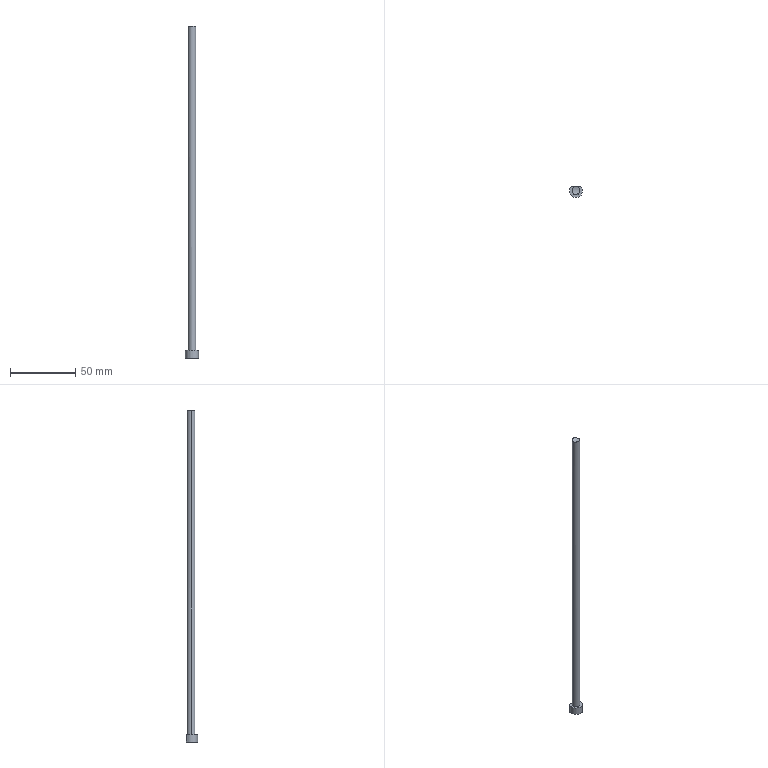Part | Creo | 1 solid | 7 faces | box 10 x 8.5 x 253.989 mm | volume 7426 mm3 | cylinder 4 | plane 3 | commonest cylinder face diameters 6 x2 10 x1 16.306 x1
STEP:
#1=CARTESIAN_POINT('',(0.,0.,0.));
#2=DIRECTION('',(0.,0.,1.));
#3=DIRECTION('',(1.,0.,0.));
#4=AXIS2_PLACEMENT_3D('',#1,#2,#3);
#5=CARTESIAN_POINT('',(228.936,8.934,-332.441));
#6=VERTEX_POINT('',#5);
#7=CARTESIAN_POINT('',(227.507,5.434,-332.441));
#8=VERTEX_POINT('',#7);
#9=CARTESIAN_POINT('',(232.507,5.434,-332.441));
#10=DIRECTION('',(0.,0.,1.));
#11=DIRECTION('',(-0.7141,0.7,0.));
#12=AXIS2_PLACEMENT_3D('',#9,#10,#11);
#13=CIRCLE('',#12,5.);
#14=EDGE_CURVE('',#6,#8,#13,.T.);
#15=ORIENTED_EDGE('',*,*,#14,.F.);
#16=CARTESIAN_POINT('',(236.078,8.934,-332.441));
#17=VERTEX_POINT('',#16);
#18=CARTESIAN_POINT('',(228.936,8.934,-332.441));
#19=DIRECTION('',(1.,0.,0.));
#20=VECTOR('',#19,7.141);
#21=LINE('',#18,#20);
#22=EDGE_CURVE('',#6,#17,#21,.T.);
#23=ORIENTED_EDGE('',*,*,#22,.T.);
#24=CARTESIAN_POINT('',(232.507,5.434,-332.441));
#25=DIRECTION('',(0.,0.,1.));
#26=DIRECTION('',(-1.,0.,0.));
#27=AXIS2_PLACEMENT_3D('',#24,#25,#26);
#28=CIRCLE('',#27,5.);
#29=EDGE_CURVE('',#8,#17,#28,.T.);
#30=ORIENTED_EDGE('',*,*,#29,.F.);
#31=EDGE_LOOP('',(#15,#23,#30));
#32=FACE_OUTER_BOUND('',#31,.F.);
#33=CARTESIAN_POINT('',(235.507,5.434,-332.441));
#34=VERTEX_POINT('',#33);
#35=CARTESIAN_POINT('',(229.507,5.434,-332.441));
#36=VERTEX_POINT('',#35);
#37=CARTESIAN_POINT('',(232.507,5.434,-332.441));
#38=DIRECTION('',(0.,0.,-1.));
#39=DIRECTION('',(1.,0.,0.));
#40=AXIS2_PLACEMENT_3D('',#37,#38,#39);
#41=CIRCLE('',#40,3.);
#42=EDGE_CURVE('',#34,#36,#41,.T.);
#43=ORIENTED_EDGE('',*,*,#42,.F.);
#44=CARTESIAN_POINT('',(232.507,5.434,-332.441));
#45=DIRECTION('',(0.,0.,-1.));
#46=DIRECTION('',(-1.,0.,0.));
#47=AXIS2_PLACEMENT_3D('',#44,#45,#46);
#48=CIRCLE('',#47,3.);
#49=EDGE_CURVE('',#36,#34,#48,.T.);
#50=ORIENTED_EDGE('',*,*,#49,.F.);
#51=EDGE_LOOP('',(#43,#50));
#52=FACE_BOUND('',#51,.F.);
#53=CARTESIAN_POINT('',(232.507,5.434,-332.441));
#54=DIRECTION('',(0.,0.,1.));
#55=DIRECTION('',(1.,0.,0.));
#56=AXIS2_PLACEMENT_3D('',#53,#54,#55);
#57=PLANE('',#56);
#58=ADVANCED_FACE('',(#32,#52),#57,.T.);
#59=ORIENTED_EDGE('',*,*,#42,.T.);
#60=CARTESIAN_POINT('',(229.507,5.434,-85.029));
#61=VERTEX_POINT('',#60);
#62=CARTESIAN_POINT('',(229.507,5.434,-332.441));
#63=DIRECTION('',(0.000000465,0.,1.));
#64=VECTOR('',#63,247.413);
#65=LINE('',#62,#64);
#66=EDGE_CURVE('',#36,#61,#65,.T.);
#67=ORIENTED_EDGE('',*,*,#66,.T.);
#68=CARTESIAN_POINT('',(235.507,5.434,-85.029));
#69=VERTEX_POINT('',#68);
#70=CARTESIAN_POINT('',(229.507,5.434,-85.029));
#71=CARTESIAN_POINT('',(229.507,5.117,-85.029));
#72=CARTESIAN_POINT('',(229.602,4.509,-84.995));
#73=CARTESIAN_POINT('',(230.037,3.641,-84.846));
#74=CARTESIAN_POINT('',(230.726,2.957,-84.654));
#75=CARTESIAN_POINT('',(231.582,2.528,-84.5));
#76=CARTESIAN_POINT('',(232.51,2.386,-84.442));
#77=CARTESIAN_POINT('',(233.434,2.53,-84.5));
#78=CARTESIAN_POINT('',(234.289,2.957,-84.654));
#79=CARTESIAN_POINT('',(234.979,3.644,-84.846));
#80=CARTESIAN_POINT('',(235.411,4.508,-84.994));
#81=CARTESIAN_POINT('',(235.507,5.116,-85.029));
#82=CARTESIAN_POINT('',(235.507,5.434,-85.029));
#83=B_SPLINE_CURVE_WITH_KNOTS('',3,(#70,#71,#72,#73,#74,#75,#76,#77,#78,#79,#80,#81,#82),.UNSPECIFIED.,.F.,.F.,(4,1,1,1,1,1,1,1,1,1,4),(0.,0.1,0.2,0.3,0.4,0.5,0.6,0.7,0.8,0.9,1.),.UNSPECIFIED.);
#84=EDGE_CURVE('',#61,#69,#83,.T.);
#85=ORIENTED_EDGE('',*,*,#84,.T.);
#86=CARTESIAN_POINT('',(235.507,5.434,-332.441));
#87=DIRECTION('',(0.,0.,1.));
#88=VECTOR('',#87,247.412);
#89=LINE('',#86,#88);
#90=EDGE_CURVE('',#34,#69,#89,.T.);
#91=ORIENTED_EDGE('',*,*,#90,.F.);
#92=EDGE_LOOP('',(#59,#67,#85,#91));
#93=FACE_OUTER_BOUND('',#92,.F.);
#94=CARTESIAN_POINT('',(232.507,5.434,-653.441));
#95=DIRECTION('',(0.,0.,1.));
#96=DIRECTION('',(1.,0.,0.));
#97=AXIS2_PLACEMENT_3D('',#94,#95,#96);
#98=CYLINDRICAL_SURFACE('',#97,3.);
#99=ADVANCED_FACE('',(#93),#98,.T.);
#100=ORIENTED_EDGE('',*,*,#49,.T.);
#101=ORIENTED_EDGE('',*,*,#90,.T.);
#102=CARTESIAN_POINT('',(235.507,5.434,-85.029));
#103=CARTESIAN_POINT('',(235.507,5.751,-85.029));
#104=CARTESIAN_POINT('',(235.411,6.36,-84.992));
#105=CARTESIAN_POINT('',(234.979,7.224,-84.842));
#106=CARTESIAN_POINT('',(234.288,7.912,-84.647));
#107=CARTESIAN_POINT('',(233.432,8.339,-84.491));
#108=CARTESIAN_POINT('',(232.509,8.481,-84.433));
#109=CARTESIAN_POINT('',(231.583,8.339,-84.491));
#110=CARTESIAN_POINT('',(230.727,7.911,-84.647));
#111=CARTESIAN_POINT('',(230.037,7.227,-84.841));
#112=CARTESIAN_POINT('',(229.602,6.359,-84.992));
#113=CARTESIAN_POINT('',(229.507,5.751,-85.028));
#114=CARTESIAN_POINT('',(229.507,5.434,-85.029));
#115=B_SPLINE_CURVE_WITH_KNOTS('',3,(#102,#103,#104,#105,#106,#107,#108,#109,#110,#111,#112,#113,#114),.UNSPECIFIED.,.F.,.F.,(4,1,1,1,1,1,1,1,1,1,4),(0.,0.1,0.2,0.3,0.4,0.5,0.6,0.7,0.8,0.9,1.),.UNSPECIFIED.);
#116=EDGE_CURVE('',#69,#61,#115,.T.);
#117=ORIENTED_EDGE('',*,*,#116,.T.);
#118=ORIENTED_EDGE('',*,*,#66,.F.);
#119=EDGE_LOOP('',(#100,#101,#117,#118));
#120=FACE_OUTER_BOUND('',#119,.F.);
#121=CARTESIAN_POINT('',(232.507,5.434,-653.441));
#122=DIRECTION('',(0.,0.,1.));
#123=DIRECTION('',(1.,0.,0.));
#124=AXIS2_PLACEMENT_3D('',#121,#122,#123);
#125=CYLINDRICAL_SURFACE('',#124,3.);
#126=ADVANCED_FACE('',(#120),#125,.T.);
#127=ORIENTED_EDGE('',*,*,#116,.F.);
#128=ORIENTED_EDGE('',*,*,#84,.F.);
#129=EDGE_LOOP('',(#127,#128));
#130=FACE_OUTER_BOUND('',#129,.F.);
#131=CARTESIAN_POINT('',(228.889,5.423,-76.876));
#132=DIRECTION('',(-1.,0.,0.));
#133=DIRECTION('',(0.,0.,1.));
#134=AXIS2_PLACEMENT_3D('',#131,#132,#133);
#135=CYLINDRICAL_SURFACE('',#134,8.153);
#136=ADVANCED_FACE('',(#130),#135,.F.);
#137=CARTESIAN_POINT('',(236.078,8.934,-338.441));
#138=VERTEX_POINT('',#137);
#139=CARTESIAN_POINT('',(236.078,8.934,-338.441));
#140=DIRECTION('',(0.,0.,1.));
#141=VECTOR('',#140,6.);
#142=LINE('',#139,#141);
#143=EDGE_CURVE('',#138,#17,#142,.T.);
#144=ORIENTED_EDGE('',*,*,#143,.F.);
#145=CARTESIAN_POINT('',(227.507,5.434,-338.441));
#146=VERTEX_POINT('',#145);
#147=CARTESIAN_POINT('',(232.507,5.434,-338.441));
#148=DIRECTION('',(0.,0.,-1.));
#149=DIRECTION('',(0.7141,0.7,0.));
#150=AXIS2_PLACEMENT_3D('',#147,#148,#149);
#151=CIRCLE('',#150,5.);
#152=EDGE_CURVE('',#138,#146,#151,.T.);
#153=ORIENTED_EDGE('',*,*,#152,.T.);
#154=CARTESIAN_POINT('',(228.936,8.934,-338.441));
#155=VERTEX_POINT('',#154);
#156=CARTESIAN_POINT('',(232.507,5.434,-338.441));
#157=DIRECTION('',(0.,0.,-1.));
#158=DIRECTION('',(-1.,0.,0.));
#159=AXIS2_PLACEMENT_3D('',#156,#157,#158);
#160=CIRCLE('',#159,5.);
#161=EDGE_CURVE('',#146,#155,#160,.T.);
#162=ORIENTED_EDGE('',*,*,#161,.T.);
#163=CARTESIAN_POINT('',(228.936,8.934,-332.441));
#164=DIRECTION('',(0.,0.,-1.));
#165=VECTOR('',#164,6.);
#166=LINE('',#163,#165);
#167=EDGE_CURVE('',#6,#155,#166,.T.);
#168=ORIENTED_EDGE('',*,*,#167,.F.);
#169=ORIENTED_EDGE('',*,*,#14,.T.);
#170=ORIENTED_EDGE('',*,*,#29,.T.);
#171=EDGE_LOOP('',(#144,#153,#162,#168,#169,#170));
#172=FACE_OUTER_BOUND('',#171,.F.);
#173=CARTESIAN_POINT('',(232.507,5.434,-332.441));
#174=DIRECTION('',(0.,0.,-1.));
#175=DIRECTION('',(-1.,0.,0.));
#176=AXIS2_PLACEMENT_3D('',#173,#174,#175);
#177=CYLINDRICAL_SURFACE('',#176,5.);
#178=ADVANCED_FACE('',(#172),#177,.T.);
#179=ORIENTED_EDGE('',*,*,#22,.F.);
#180=ORIENTED_EDGE('',*,*,#167,.T.);
#181=CARTESIAN_POINT('',(228.936,8.934,-338.441));
#182=DIRECTION('',(1.,0.,0.));
#183=VECTOR('',#182,7.141);
#184=LINE('',#181,#183);
#185=EDGE_CURVE('',#155,#138,#184,.T.);
#186=ORIENTED_EDGE('',*,*,#185,.T.);
#187=ORIENTED_EDGE('',*,*,#143,.T.);
#188=EDGE_LOOP('',(#179,#180,#186,#187));
#189=FACE_OUTER_BOUND('',#188,.F.);
#190=CARTESIAN_POINT('',(232.507,8.934,-338.441));
#191=DIRECTION('',(0.,1.,0.));
#192=DIRECTION('',(0.,0.,1.));
#193=AXIS2_PLACEMENT_3D('',#190,#191,#192);
#194=PLANE('',#193);
#195=ADVANCED_FACE('',(#189),#194,.T.);
#196=ORIENTED_EDGE('',*,*,#185,.F.);
#197=ORIENTED_EDGE('',*,*,#161,.F.);
#198=ORIENTED_EDGE('',*,*,#152,.F.);
#199=EDGE_LOOP('',(#196,#197,#198));
#200=FACE_OUTER_BOUND('',#199,.F.);
#201=CARTESIAN_POINT('',(232.507,5.434,-338.441));
#202=DIRECTION('',(0.,0.,1.));
#203=DIRECTION('',(1.,0.,0.));
#204=AXIS2_PLACEMENT_3D('',#201,#202,#203);
#205=PLANE('',#204);
#206=ADVANCED_FACE('',(#200),#205,.F.);
#207=CLOSED_SHELL('',(#58,#99,#126,#136,#178,#195,#206));
#208=MANIFOLD_SOLID_BREP('',#207);
#209=(LENGTH_UNIT()NAMED_UNIT(*)SI_UNIT(.MILLI.,.METRE.));
#210=UNCERTAINTY_MEASURE_WITH_UNIT(LENGTH_MEASURE(0.02543),#209,'','');
#211=(NAMED_UNIT(*)PLANE_ANGLE_UNIT()SI_UNIT($,.RADIAN.));
#212=PLANE_ANGLE_MEASURE_WITH_UNIT(PLANE_ANGLE_MEASURE(0.01745),#211);
#213=(CONVERSION_BASED_UNIT('DEGREE',#212)NAMED_UNIT(*)PLANE_ANGLE_UNIT());
#214=(NAMED_UNIT(*)SI_UNIT($,.STERADIAN.)SOLID_ANGLE_UNIT());
#215=(GEOMETRIC_REPRESENTATION_CONTEXT(3)GLOBAL_UNCERTAINTY_ASSIGNED_CONTEXT((#210))GLOBAL_UNIT_ASSIGNED_CONTEXT((#209,#213,#214))REPRESENTATION_CONTEXT('',''));
#216=ADVANCED_BREP_SHAPE_REPRESENTATION('',(#4,#208),#215);